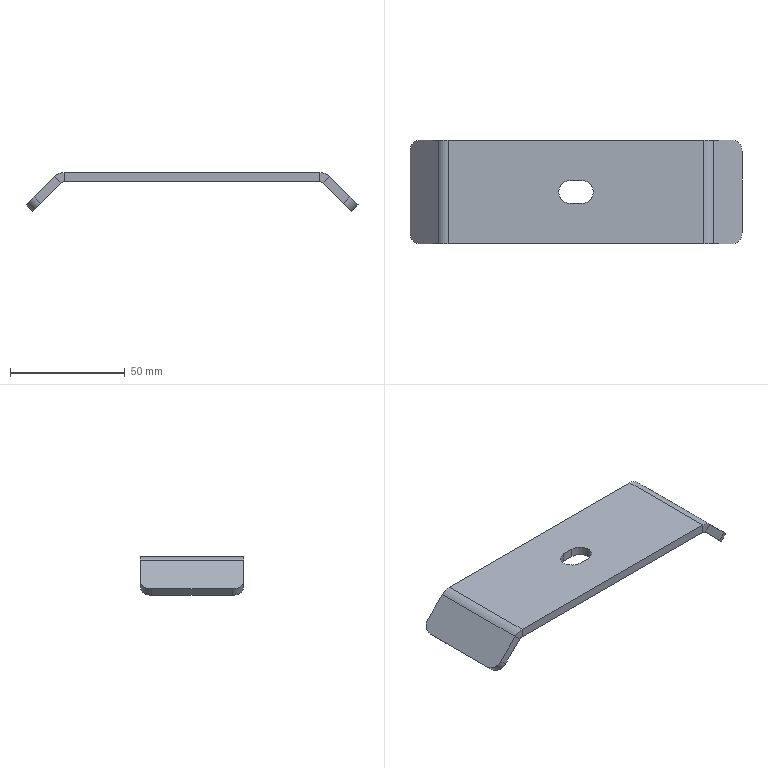Part | STEP file | PN_0073 guardrail connecting plate (spacing 100)_Default<As Machined> | 1 solid | 30 faces | box 144.912 x 45 x 17 mm | volume 26939 mm3 | plane 20 | cylinder 10 | commonest cylinder face diameters 10 x6 4 x2 12 x2